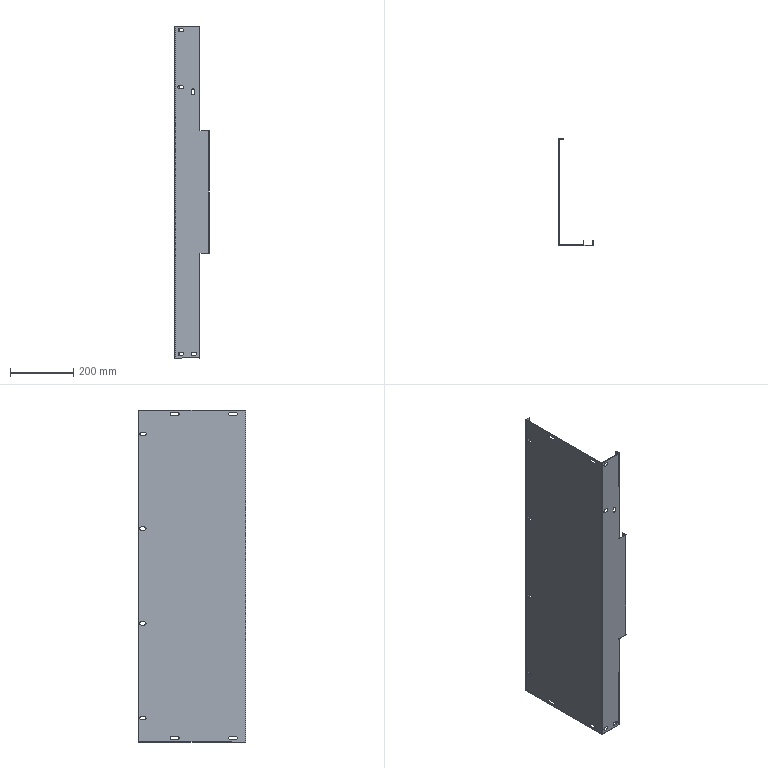Part | SolidWorks | features ICE 11, Cut 5, EdgeFlange 5, SMBaseFlange 5, Chamfer 1, FlatPattern 1, LPattern 1, SheetMetal 1 | 1 solid | 135 faces | box 110 x 339.5 x 1050 mm | volume 713005 mm3 | plane 90 | cylinder 45 | commonest cylinder face diameters 10 x18 9 x12 0.4 x5 3.4 x5 11 x5